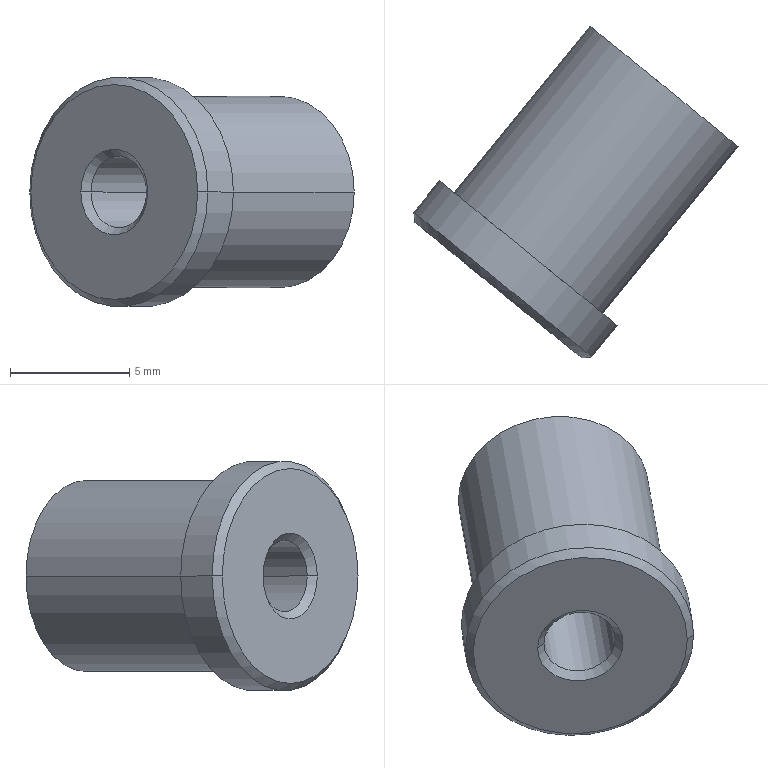Part | SolidWorks | features BaseBody 1 | 1 solid | 13 faces | box 13.578 x 13.897 x 9.6 mm | volume 517.614 mm3 | cylinder 6 | cone 4 | plane 3 | commonest cylinder face diameters 3 x2 8 x2 9.6 x2
STEP:
#1=CARTESIAN_POINT('',(534.69,-155.958,299.195));
#2=VERTEX_POINT('',#1);
#3=CARTESIAN_POINT('',(528.483,-150.91,299.195));
#4=VERTEX_POINT('',#3);
#5=CARTESIAN_POINT('',(531.587,-153.434,299.195));
#6=DIRECTION('',(-0.6309,-0.7758,0.000000012));
#7=DIRECTION('',(0.7758,-0.6309,0.));
#8=AXIS2_PLACEMENT_3D('',#5,#6,#7);
#9=CIRCLE('',#8,4.);
#10=EDGE_CURVE('',#2,#4,#9,.T.);
#11=ORIENTED_EDGE('',*,*,#10,.T.);
#12=CARTESIAN_POINT('',(522.805,-157.893,299.195));
#13=VERTEX_POINT('',#12);
#14=CARTESIAN_POINT('',(522.805,-157.893,299.195));
#15=DIRECTION('',(-0.6309,-0.7758,0.000000012));
#16=VECTOR('',#15,1000.);
#17=LINE('',#14,#16);
#18=EDGE_CURVE('',#4,#13,#17,.T.);
#19=ORIENTED_EDGE('',*,*,#18,.T.);
#20=CARTESIAN_POINT('',(529.012,-162.94,299.195));
#21=VERTEX_POINT('',#20);
#22=CARTESIAN_POINT('',(525.908,-160.417,299.195));
#23=DIRECTION('',(0.6309,0.7758,-0.000000012));
#24=DIRECTION('',(0.7758,-0.6309,0.));
#25=AXIS2_PLACEMENT_3D('',#22,#23,#24);
#26=CIRCLE('',#25,4.);
#27=EDGE_CURVE('',#13,#21,#26,.T.);
#28=ORIENTED_EDGE('',*,*,#27,.T.);
#29=CARTESIAN_POINT('',(529.012,-162.94,299.195));
#30=DIRECTION('',(-0.6309,-0.7758,0.000000012));
#31=VECTOR('',#30,1000.);
#32=LINE('',#29,#31);
#33=EDGE_CURVE('',#2,#21,#32,.T.);
#34=ORIENTED_EDGE('',*,*,#33,.F.);
#35=EDGE_LOOP('',(#11,#19,#28,#34));
#36=FACE_OUTER_BOUND('',#35,.T.);
#37=CARTESIAN_POINT('',(525.908,-160.417,299.195));
#38=DIRECTION('',(-0.6309,-0.7758,0.000000012));
#39=DIRECTION('',(0.7758,-0.6309,0.));
#40=AXIS2_PLACEMENT_3D('',#37,#38,#39);
#41=CYLINDRICAL_SURFACE('',#40,4.);
#42=ADVANCED_FACE('',(#36),#41,.T.);
#43=CARTESIAN_POINT('',(526.,-162.682,299.195));
#44=VERTEX_POINT('',#43);
#45=CARTESIAN_POINT('',(523.672,-160.789,299.195));
#46=VERTEX_POINT('',#45);
#47=CARTESIAN_POINT('',(524.836,-161.736,299.195));
#48=DIRECTION('',(0.6309,0.7758,-0.000000012));
#49=DIRECTION('',(-0.7758,0.6309,0.));
#50=AXIS2_PLACEMENT_3D('',#47,#48,#49);
#51=CIRCLE('',#50,1.5);
#52=EDGE_CURVE('',#44,#46,#51,.T.);
#53=ORIENTED_EDGE('',*,*,#52,.F.);
#54=CARTESIAN_POINT('',(532.751,-154.38,299.195));
#55=VERTEX_POINT('',#54);
#56=CARTESIAN_POINT('',(532.751,-154.38,299.195));
#57=DIRECTION('',(0.6309,0.7758,-0.000000012));
#58=VECTOR('',#57,1000.);
#59=LINE('',#56,#58);
#60=EDGE_CURVE('',#44,#55,#59,.T.);
#61=ORIENTED_EDGE('',*,*,#60,.T.);
#62=CARTESIAN_POINT('',(530.423,-152.488,299.195));
#63=VERTEX_POINT('',#62);
#64=CARTESIAN_POINT('',(531.587,-153.434,299.195));
#65=DIRECTION('',(-0.6309,-0.7758,0.000000012));
#66=DIRECTION('',(-0.7758,0.6309,0.));
#67=AXIS2_PLACEMENT_3D('',#64,#65,#66);
#68=CIRCLE('',#67,1.5);
#69=EDGE_CURVE('',#63,#55,#68,.T.);
#70=ORIENTED_EDGE('',*,*,#69,.F.);
#71=CARTESIAN_POINT('',(530.423,-152.488,299.195));
#72=DIRECTION('',(0.6309,0.7758,-0.000000012));
#73=VECTOR('',#72,1000.);
#74=LINE('',#71,#73);
#75=EDGE_CURVE('',#46,#63,#74,.T.);
#76=ORIENTED_EDGE('',*,*,#75,.F.);
#77=EDGE_LOOP('',(#53,#61,#70,#76));
#78=FACE_OUTER_BOUND('',#77,.T.);
#79=CARTESIAN_POINT('',(531.587,-153.434,299.195));
#80=DIRECTION('',(0.6309,0.7758,-0.000000012));
#81=DIRECTION('',(-0.7758,0.6309,0.));
#82=AXIS2_PLACEMENT_3D('',#79,#80,#81);
#83=CYLINDRICAL_SURFACE('',#82,1.5);
#84=ADVANCED_FACE('',(#78),#83,.F.);
#85=CARTESIAN_POINT('',(521.112,-158.707,299.195));
#86=VERTEX_POINT('',#85);
#87=CARTESIAN_POINT('',(528.56,-164.764,299.195));
#88=VERTEX_POINT('',#87);
#89=CARTESIAN_POINT('',(524.836,-161.736,299.195));
#90=DIRECTION('',(0.6309,0.7758,-0.000000012));
#91=DIRECTION('',(-0.7758,0.6309,0.));
#92=AXIS2_PLACEMENT_3D('',#89,#90,#91);
#93=CIRCLE('',#92,4.8);
#94=EDGE_CURVE('',#86,#88,#93,.T.);
#95=ORIENTED_EDGE('',*,*,#94,.T.);
#96=CARTESIAN_POINT('',(529.633,-163.445,299.195));
#97=VERTEX_POINT('',#96);
#98=CARTESIAN_POINT('',(529.633,-163.445,299.195));
#99=DIRECTION('',(0.6309,0.7758,-0.000000012));
#100=VECTOR('',#99,1000.);
#101=LINE('',#98,#100);
#102=EDGE_CURVE('',#88,#97,#101,.T.);
#103=ORIENTED_EDGE('',*,*,#102,.T.);
#104=CARTESIAN_POINT('',(522.184,-157.388,299.195));
#105=VERTEX_POINT('',#104);
#106=CARTESIAN_POINT('',(525.908,-160.417,299.195));
#107=DIRECTION('',(-0.6309,-0.7758,0.000000012));
#108=DIRECTION('',(-0.7758,0.6309,0.));
#109=AXIS2_PLACEMENT_3D('',#106,#107,#108);
#110=CIRCLE('',#109,4.8);
#111=EDGE_CURVE('',#97,#105,#110,.T.);
#112=ORIENTED_EDGE('',*,*,#111,.T.);
#113=CARTESIAN_POINT('',(522.184,-157.388,299.195));
#114=DIRECTION('',(0.6309,0.7758,-0.000000012));
#115=VECTOR('',#114,1000.);
#116=LINE('',#113,#115);
#117=EDGE_CURVE('',#86,#105,#116,.T.);
#118=ORIENTED_EDGE('',*,*,#117,.F.);
#119=EDGE_LOOP('',(#95,#103,#112,#118));
#120=FACE_OUTER_BOUND('',#119,.T.);
#121=CARTESIAN_POINT('',(525.908,-160.417,299.195));
#122=DIRECTION('',(0.6309,0.7758,-0.000000012));
#123=DIRECTION('',(-0.7758,0.6309,0.));
#124=AXIS2_PLACEMENT_3D('',#121,#122,#123);
#125=CYLINDRICAL_SURFACE('',#124,4.8);
#126=ADVANCED_FACE('',(#120),#125,.T.);
#127=ORIENTED_EDGE('',*,*,#52,.T.);
#128=CARTESIAN_POINT('',(523.25,-160.833,299.195));
#129=VERTEX_POINT('',#128);
#130=CARTESIAN_POINT('',(523.25,-160.833,299.195));
#131=DIRECTION('',(-0.9947,-0.1025,0.000000009));
#132=VECTOR('',#131,1000.);
#133=LINE('',#130,#132);
#134=EDGE_CURVE('',#46,#129,#133,.T.);
#135=ORIENTED_EDGE('',*,*,#134,.T.);
#136=CARTESIAN_POINT('',(526.043,-163.104,299.195));
#137=VERTEX_POINT('',#136);
#138=CARTESIAN_POINT('',(524.647,-161.968,299.195));
#139=DIRECTION('',(0.6309,0.7758,-0.000000012));
#140=DIRECTION('',(0.7758,-0.6309,0.));
#141=AXIS2_PLACEMENT_3D('',#138,#139,#140);
#142=CIRCLE('',#141,1.8);
#143=EDGE_CURVE('',#137,#129,#142,.T.);
#144=ORIENTED_EDGE('',*,*,#143,.F.);
#145=CARTESIAN_POINT('',(526.043,-163.104,299.195));
#146=DIRECTION('',(0.1025,-0.9947,0.000000009));
#147=VECTOR('',#146,1000.);
#148=LINE('',#145,#147);
#149=EDGE_CURVE('',#44,#137,#148,.T.);
#150=ORIENTED_EDGE('',*,*,#149,.F.);
#151=EDGE_LOOP('',(#127,#135,#144,#150));
#152=FACE_OUTER_BOUND('',#151,.T.);
#153=CARTESIAN_POINT('',(524.647,-161.968,299.195));
#154=DIRECTION('',(-0.6309,-0.7758,0.000000012));
#155=DIRECTION('',(0.7758,-0.6309,0.));
#156=AXIS2_PLACEMENT_3D('',#153,#154,#155);
#157=CONICAL_SURFACE('',#156,1.8,0.7854);
#158=ADVANCED_FACE('',(#152),#157,.F.);
#159=CARTESIAN_POINT('',(521.155,-159.129,299.195));
#160=VERTEX_POINT('',#159);
#161=CARTESIAN_POINT('',(528.138,-164.807,299.195));
#162=VERTEX_POINT('',#161);
#163=CARTESIAN_POINT('',(524.647,-161.968,299.195));
#164=DIRECTION('',(0.6309,0.7758,-0.000000012));
#165=DIRECTION('',(-0.7758,0.6309,0.));
#166=AXIS2_PLACEMENT_3D('',#163,#164,#165);
#167=CIRCLE('',#166,4.5);
#168=EDGE_CURVE('',#160,#162,#167,.T.);
#169=ORIENTED_EDGE('',*,*,#168,.T.);
#170=CARTESIAN_POINT('',(528.56,-164.764,299.195));
#171=DIRECTION('',(0.9947,0.1025,-0.000000009));
#172=VECTOR('',#171,1000.);
#173=LINE('',#170,#172);
#174=EDGE_CURVE('',#162,#88,#173,.T.);
#175=ORIENTED_EDGE('',*,*,#174,.T.);
#176=ORIENTED_EDGE('',*,*,#94,.F.);
#177=CARTESIAN_POINT('',(521.112,-158.707,299.195));
#178=DIRECTION('',(-0.1025,0.9947,-0.000000009));
#179=VECTOR('',#178,1000.);
#180=LINE('',#177,#179);
#181=EDGE_CURVE('',#160,#86,#180,.T.);
#182=ORIENTED_EDGE('',*,*,#181,.F.);
#183=EDGE_LOOP('',(#169,#175,#176,#182));
#184=FACE_OUTER_BOUND('',#183,.T.);
#185=CARTESIAN_POINT('',(524.836,-161.736,299.195));
#186=DIRECTION('',(0.6309,0.7758,-0.000000012));
#187=DIRECTION('',(-0.7758,0.6309,0.));
#188=AXIS2_PLACEMENT_3D('',#185,#186,#187);
#189=CONICAL_SURFACE('',#188,4.8,0.7854);
#190=ADVANCED_FACE('',(#184),#189,.T.);
#191=ORIENTED_EDGE('',*,*,#18,.F.);
#192=CARTESIAN_POINT('',(531.587,-153.434,299.195));
#193=DIRECTION('',(-0.6309,-0.7758,0.000000012));
#194=DIRECTION('',(0.7758,-0.6309,0.));
#195=AXIS2_PLACEMENT_3D('',#192,#193,#194);
#196=CIRCLE('',#195,4.);
#197=EDGE_CURVE('',#4,#2,#196,.T.);
#198=ORIENTED_EDGE('',*,*,#197,.T.);
#199=ORIENTED_EDGE('',*,*,#33,.T.);
#200=CARTESIAN_POINT('',(525.908,-160.417,299.195));
#201=DIRECTION('',(0.6309,0.7758,-0.000000012));
#202=DIRECTION('',(0.7758,-0.6309,0.));
#203=AXIS2_PLACEMENT_3D('',#200,#201,#202);
#204=CIRCLE('',#203,4.);
#205=EDGE_CURVE('',#21,#13,#204,.T.);
#206=ORIENTED_EDGE('',*,*,#205,.T.);
#207=EDGE_LOOP('',(#191,#198,#199,#206));
#208=FACE_OUTER_BOUND('',#207,.T.);
#209=CARTESIAN_POINT('',(525.908,-160.417,299.195));
#210=DIRECTION('',(-0.6309,-0.7758,0.000000012));
#211=DIRECTION('',(0.7758,-0.6309,0.));
#212=AXIS2_PLACEMENT_3D('',#209,#210,#211);
#213=CYLINDRICAL_SURFACE('',#212,4.);
#214=ADVANCED_FACE('',(#208),#213,.T.);
#215=ORIENTED_EDGE('',*,*,#10,.F.);
#216=ORIENTED_EDGE('',*,*,#197,.F.);
#217=EDGE_LOOP('',(#215,#216));
#218=FACE_OUTER_BOUND('',#217,.T.);
#219=ORIENTED_EDGE('',*,*,#69,.T.);
#220=CARTESIAN_POINT('',(531.587,-153.434,299.195));
#221=DIRECTION('',(-0.6309,-0.7758,0.000000012));
#222=DIRECTION('',(-0.7758,0.6309,0.));
#223=AXIS2_PLACEMENT_3D('',#220,#221,#222);
#224=CIRCLE('',#223,1.5);
#225=EDGE_CURVE('',#55,#63,#224,.T.);
#226=ORIENTED_EDGE('',*,*,#225,.T.);
#227=EDGE_LOOP('',(#219,#226));
#228=FACE_BOUND('',#227,.T.);
#229=CARTESIAN_POINT('',(531.587,-153.434,299.195));
#230=DIRECTION('',(0.6309,0.7758,-0.000000012));
#231=DIRECTION('',(-0.7758,0.6309,0.));
#232=AXIS2_PLACEMENT_3D('',#229,#230,#231);
#233=PLANE('',#232);
#234=ADVANCED_FACE('',(#218,#228),#233,.T.);
#235=CARTESIAN_POINT('',(525.908,-160.417,299.195));
#236=DIRECTION('',(-0.6309,-0.7758,0.000000012));
#237=DIRECTION('',(-0.7758,0.6309,0.));
#238=AXIS2_PLACEMENT_3D('',#235,#236,#237);
#239=CIRCLE('',#238,4.8);
#240=EDGE_CURVE('',#105,#97,#239,.T.);
#241=ORIENTED_EDGE('',*,*,#240,.F.);
#242=ORIENTED_EDGE('',*,*,#111,.F.);
#243=EDGE_LOOP('',(#241,#242));
#244=FACE_OUTER_BOUND('',#243,.T.);
#245=ORIENTED_EDGE('',*,*,#205,.F.);
#246=ORIENTED_EDGE('',*,*,#27,.F.);
#247=EDGE_LOOP('',(#245,#246));
#248=FACE_BOUND('',#247,.T.);
#249=CARTESIAN_POINT('',(525.908,-160.417,299.195));
#250=DIRECTION('',(-0.6309,-0.7758,0.000000012));
#251=DIRECTION('',(0.7758,-0.6309,0.));
#252=AXIS2_PLACEMENT_3D('',#249,#250,#251);
#253=PLANE('',#252);
#254=ADVANCED_FACE('',(#244,#248),#253,.F.);
#255=ORIENTED_EDGE('',*,*,#60,.F.);
#256=CARTESIAN_POINT('',(524.836,-161.736,299.195));
#257=DIRECTION('',(0.6309,0.7758,-0.000000012));
#258=DIRECTION('',(-0.7758,0.6309,0.));
#259=AXIS2_PLACEMENT_3D('',#256,#257,#258);
#260=CIRCLE('',#259,1.5);
#261=EDGE_CURVE('',#46,#44,#260,.T.);
#262=ORIENTED_EDGE('',*,*,#261,.F.);
#263=ORIENTED_EDGE('',*,*,#75,.T.);
#264=ORIENTED_EDGE('',*,*,#225,.F.);
#265=EDGE_LOOP('',(#255,#262,#263,#264));
#266=FACE_OUTER_BOUND('',#265,.T.);
#267=CARTESIAN_POINT('',(531.587,-153.434,299.195));
#268=DIRECTION('',(0.6309,0.7758,-0.000000012));
#269=DIRECTION('',(-0.7758,0.6309,0.));
#270=AXIS2_PLACEMENT_3D('',#267,#268,#269);
#271=CYLINDRICAL_SURFACE('',#270,1.5);
#272=ADVANCED_FACE('',(#266),#271,.F.);
#273=ORIENTED_EDGE('',*,*,#102,.F.);
#274=CARTESIAN_POINT('',(524.836,-161.736,299.195));
#275=DIRECTION('',(0.6309,0.7758,-0.000000012));
#276=DIRECTION('',(-0.7758,0.6309,0.));
#277=AXIS2_PLACEMENT_3D('',#274,#275,#276);
#278=CIRCLE('',#277,4.8);
#279=EDGE_CURVE('',#88,#86,#278,.T.);
#280=ORIENTED_EDGE('',*,*,#279,.T.);
#281=ORIENTED_EDGE('',*,*,#117,.T.);
#282=ORIENTED_EDGE('',*,*,#240,.T.);
#283=EDGE_LOOP('',(#273,#280,#281,#282));
#284=FACE_OUTER_BOUND('',#283,.T.);
#285=CARTESIAN_POINT('',(525.908,-160.417,299.195));
#286=DIRECTION('',(0.6309,0.7758,-0.000000012));
#287=DIRECTION('',(-0.7758,0.6309,0.));
#288=AXIS2_PLACEMENT_3D('',#285,#286,#287);
#289=CYLINDRICAL_SURFACE('',#288,4.8);
#290=ADVANCED_FACE('',(#284),#289,.T.);
#291=ORIENTED_EDGE('',*,*,#134,.F.);
#292=ORIENTED_EDGE('',*,*,#261,.T.);
#293=ORIENTED_EDGE('',*,*,#149,.T.);
#294=CARTESIAN_POINT('',(524.647,-161.968,299.195));
#295=DIRECTION('',(0.6309,0.7758,-0.000000012));
#296=DIRECTION('',(0.7758,-0.6309,0.));
#297=AXIS2_PLACEMENT_3D('',#294,#295,#296);
#298=CIRCLE('',#297,1.8);
#299=EDGE_CURVE('',#129,#137,#298,.T.);
#300=ORIENTED_EDGE('',*,*,#299,.F.);
#301=EDGE_LOOP('',(#291,#292,#293,#300));
#302=FACE_OUTER_BOUND('',#301,.T.);
#303=CARTESIAN_POINT('',(524.647,-161.968,299.195));
#304=DIRECTION('',(-0.6309,-0.7758,0.000000012));
#305=DIRECTION('',(0.7758,-0.6309,0.));
#306=AXIS2_PLACEMENT_3D('',#303,#304,#305);
#307=CONICAL_SURFACE('',#306,1.8,0.7854);
#308=ADVANCED_FACE('',(#302),#307,.F.);
#309=ORIENTED_EDGE('',*,*,#174,.F.);
#310=CARTESIAN_POINT('',(524.647,-161.968,299.195));
#311=DIRECTION('',(0.6309,0.7758,-0.000000012));
#312=DIRECTION('',(-0.7758,0.6309,0.));
#313=AXIS2_PLACEMENT_3D('',#310,#311,#312);
#314=CIRCLE('',#313,4.5);
#315=EDGE_CURVE('',#162,#160,#314,.T.);
#316=ORIENTED_EDGE('',*,*,#315,.T.);
#317=ORIENTED_EDGE('',*,*,#181,.T.);
#318=ORIENTED_EDGE('',*,*,#279,.F.);
#319=EDGE_LOOP('',(#309,#316,#317,#318));
#320=FACE_OUTER_BOUND('',#319,.T.);
#321=CARTESIAN_POINT('',(524.836,-161.736,299.195));
#322=DIRECTION('',(0.6309,0.7758,-0.000000012));
#323=DIRECTION('',(-0.7758,0.6309,0.));
#324=AXIS2_PLACEMENT_3D('',#321,#322,#323);
#325=CONICAL_SURFACE('',#324,4.8,0.7854);
#326=ADVANCED_FACE('',(#320),#325,.T.);
#327=ORIENTED_EDGE('',*,*,#143,.T.);
#328=ORIENTED_EDGE('',*,*,#299,.T.);
#329=EDGE_LOOP('',(#327,#328));
#330=FACE_BOUND('',#329,.T.);
#331=ORIENTED_EDGE('',*,*,#168,.F.);
#332=ORIENTED_EDGE('',*,*,#315,.F.);
#333=EDGE_LOOP('',(#331,#332));
#334=FACE_OUTER_BOUND('',#333,.T.);
#335=CARTESIAN_POINT('',(524.647,-161.968,299.195));
#336=DIRECTION('',(-0.6309,-0.7758,0.000000012));
#337=DIRECTION('',(0.7758,-0.6309,0.));
#338=AXIS2_PLACEMENT_3D('',#335,#336,#337);
#339=PLANE('',#338);
#340=ADVANCED_FACE('',(#330,#334),#339,.T.);
#341=CLOSED_SHELL('',(#42,#84,#126,#158,#190,#214,#234,#254,#272,#290,#308,#326,#340));
#342=MANIFOLD_SOLID_BREP('',#341);
#343=CARTESIAN_POINT('',(0.,0.,0.));
#344=DIRECTION('',(0.,0.,1.));
#345=DIRECTION('',(1.,0.,0.));
#346=AXIS2_PLACEMENT_3D('',#343,#344,#345);
#347=(LENGTH_UNIT()NAMED_UNIT(*)SI_UNIT(.MILLI.,.METRE.));
#348=UNCERTAINTY_MEASURE_WITH_UNIT(LENGTH_MEASURE(0.00001),#347,'','');
#349=(NAMED_UNIT(*)PLANE_ANGLE_UNIT()SI_UNIT($,.RADIAN.));
#350=(NAMED_UNIT(*)SI_UNIT($,.STERADIAN.)SOLID_ANGLE_UNIT());
#351=(GEOMETRIC_REPRESENTATION_CONTEXT(3)GLOBAL_UNCERTAINTY_ASSIGNED_CONTEXT((#348))GLOBAL_UNIT_ASSIGNED_CONTEXT((#347,#349,#350))REPRESENTATION_CONTEXT('',''));
#352=ADVANCED_BREP_SHAPE_REPRESENTATION('',(#342,#346),#351);